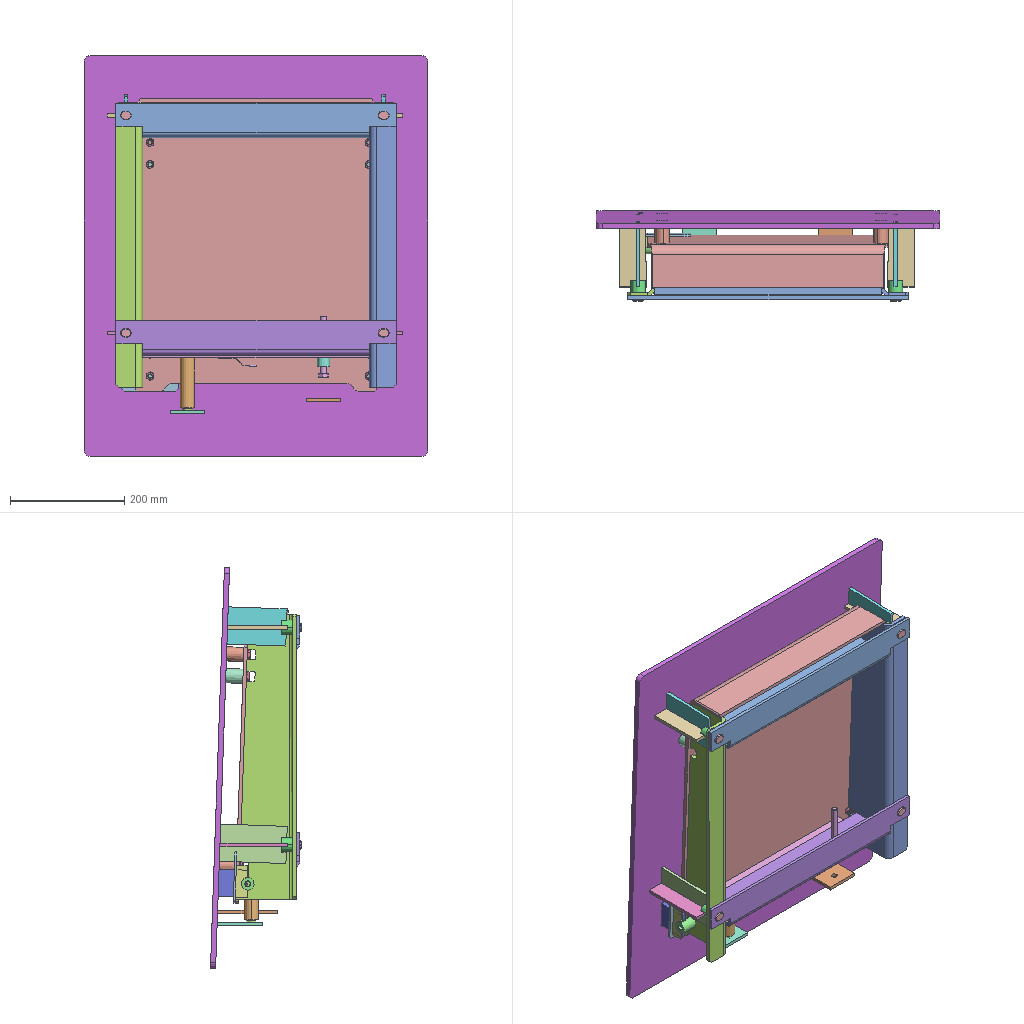Assembly | SolidWorks | 27 different items | 53 placed | box 600 x 159 x 700 mm
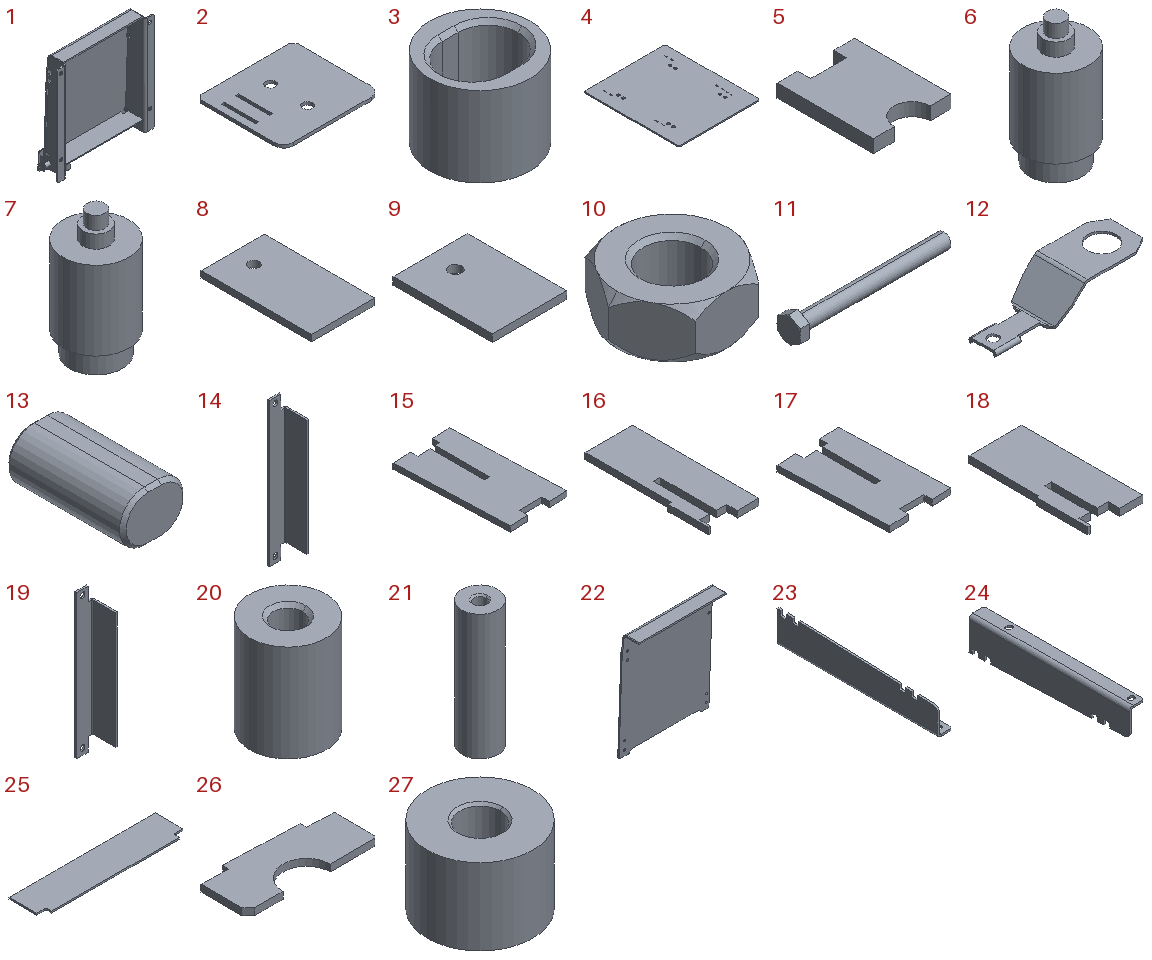Parts list (item | name | quantity | parent item | size | volume | features):
1 | (subassembly) | x1 | - | 490 x 110.428 x 539.749 mm | 2418391 mm3 | features ReferencePattern 8, LocalLPattern 4, InContextFeatHolder 2, Cut 1
2 | - | x1 | in 1 | 100 x 90 x 3.2 mm | 27363 mm3 | features FlatPattern 1, SMBaseFlange 1, SheetMetal 1
3 | - | x4 | - | 25 x 25 x 20 mm | 5055 mm3 | features Chamfer 1, Extrusion 1
4 | - | x1 | - | 600 x 700 x 9 mm | 3746150 mm3 | features Cut 3, LPattern 2, Extrusion 1, Fillet 1
5 | - | x1 | - | 47.495 x 59 x 8 mm | 19489 mm3 | features Extrusion 1
6 | - | x3 | - | 25 x 25 x 48 mm | 17814 mm3 | features ICE 3, Extrusion 1
7 | - | x5 | - | 25 x 25 x 48 mm | 17814 mm3 | features ICE 3, Extrusion 1
8 | - | x1 | - | 60 x 104.7 x 6 mm | 37221 mm3 | features FlatPattern 1, SMBaseFlange 1, SheetMetal 1
9 | - | x1 | - | 60 x 79.5 x 6 mm | 28149 mm3 | features FlatPattern 1, SMBaseFlange 1, SheetMetal 1
10 | - | x8 | in 1 | 15.011 x 13.013 x 6 mm | 641.329 mm3 | features RevCut 3, Chamfer 2, Extrusion 1, RefAxis 1
11 | - | x2 | - | 107.08 x 15.73 x 18.163 mm | 9342 mm3 | features RevCut 2, Boss 1, Chamfer 1, Extrusion 1, Fillet 1, LPattern 1, Revolution 1
12 | - | x2 | in 1 | 66.449 x 23 x 15.525 mm | 1224 mm3 | features ICE 6, EdgeFlange 2, Hem 2, FlatPattern 1, SMBaseFlange 1, SheetMetal 1
13 | - | x4 | - | 19 x 35 x 15 mm | 8232 mm3 | features Chamfer 1, Extrusion 1
14 | - | x1 | - | 60 x 80 x 490 mm | 331985 mm3 | features ICE 2, FlatPattern 1, SMBaseFlange 1, SheetMetal 1
15 | - | x2 | - | 69.342 x 126.628 x 6 mm | 43791 mm3 | features Extrusion 1, ICE 1
16 | - | x2 | - | 47.002 x 117.5 x 6 mm | 28307 mm3 | features ICE 2, Extrusion 1
17 | - | x2 | - | 68.823 x 113.082 x 6 mm | 38487 mm3 | features Extrusion 1, ICE 1
18 | - | x2 | - | 47.5 x 103.96 x 6 mm | 26008 mm3 | features ICE 2, Extrusion 1
19 | - | x1 | - | 60 x 85 x 490 mm | 343865 mm3 | features ICE 2, FlatPattern 1, SMBaseFlange 1, SheetMetal 1
20 | - | x1 | in 1 | 22 x 22 x 28 mm | 9040 mm3 | features Chamfer 1, Extrusion 1, Helix 1, ICE 1
21 | - | x1 | in 1 | 25 x 25 x 87 mm | 41273 mm3 | features Chamfer 1, Extrusion 1, Helix 1, ICE 1
22 | - | x1 | in 1 | 420 x 93.297 x 511.152 mm | 1409801 mm3 | features Cut 1, FlatPattern 1, SM3dBend 1, SMBaseFlange 1, SheetMetal 1
23 | - | x1 | in 1 | 47 x 498.4 x 101 mm | 376827 mm3 | features ICE 4, Chamfer 1, EdgeFlange 1, Fillet 1, FlatPattern 1, SMBaseFlange 1, SheetMetal 1
24 | - | x1 | in 1 | 47 x 498.4 x 101 mm | 376827 mm3 | features ICE 3, Fillet 2, Chamfer 1, EdgeFlange 1, FlatPattern 1, SMBaseFlange 1, SheetMetal 1
25 | - | x1 | in 1 | 396 x 90 x 4.5 mm | 157053 mm3 | features FlatPattern 1, SMBaseFlange 1, SheetMetal 1
26 | - | x2 | in 1 | 60 x 24.545 x 3.2 mm | 3731 mm3 | features FlatPattern 1, SMBaseFlange 1, SheetMetal 1
27 | - | x1 | in 1 | 22 x 22 x 16 mm | 5167 mm3 | features Chamfer 1, Extrusion 1, ICE 1
Mates (type | each side: item.copy, entity, surface, feature):
In the top assembly
Parallel | 22.1 face plane Base-Flange1 | 4.1 face plane Boss-Extrude1
Parallel | 22.1 face plane Sketched Bend1 | 4.1 face plane Boss-Extrude1
DistanceDim | 4.1 face plane Boss-Extrude1 | 22.1 face plane Sketched Bend1
DistanceDim | 4.1 face plane Boss-Extrude1 | 22.1 face plane Base-Flange1 | 2 times
Concentric | 4.1 face cylinder Cut-Extrude2 | 7.1 face cylinder Boss-Extrude3
Coincident | 4.1 face plane Boss-Extrude1 | 7.1 face plane Boss-Extrude3
Concentric | 4.1 face cylinder Cut-Extrude2 | 6.1 face cylinder Boss-Extrude3
Coincident | 4.1 face plane Boss-Extrude1 | 6.1 face plane Boss-Extrude3
Concentric | 4.1 face cylinder Cut-Extrude2 | 6.2 face cylinder Boss-Extrude3
Coincident | 4.1 face plane Boss-Extrude1 | 6.2 face plane Boss-Extrude3
Concentric | 4.1 face cylinder Cut-Extrude2 | 6.3 face cylinder Boss-Extrude3
Coincident | 4.1 face plane Boss-Extrude1 | 6.3 face plane Boss-Extrude3
DistanceDim | 20.1 face plane Boss-Extrude1 | 5.1 face plane Boss-Extrude1
Concentric | 20.1 face cylinder Boss-Extrude1 | 5.1 face cylinder Boss-Extrude1
Parallel | 5.1 face plane Boss-Extrude1 | 4.1 face plane Boss-Extrude1
Parallel | 23.1 face plane Base-Flange1 | 15.1 face plane Boss-Extrude1
Parallel | 23.1 face plane Edge-Flange1 | 15.1 face plane Cut-Extrude1
Coincident | 15.1 face plane Cut-Extrude1 | 16.1 face plane Boss-Extrude1
Coincident | 15.1 face plane Boss-Extrude1 | 16.1 face plane Cut-Extrude1
Coincident | 4.1 face plane LPattern4 | 17.1 face plane Boss-Extrude1 | 2 times
Coincident | 17.1 face plane Cut-Extrude1 | 18.1 face plane Boss-Extrude1
Coincident | 17.1 face plane Boss-Extrude1 | 18.1 edge
Coincident | 4.1 face plane LPattern5 | 15.2 edge
Coincident | 4.1 face plane LPattern5 | 15.2 face plane Boss-Extrude1
Coincident | 15.2 face plane Boss-Extrude1 | 16.2 edge
Coincident | 15.2 edge | 16.2 face plane Boss-Extrude1 | 2 times
Coincident | 15.2 face plane Boss-Extrude1 | 16.2 face plane Cut-Extrude1
Coincident | 4.1 face plane LPattern5 | 17.2 face plane Boss-Extrude1 | 2 times
Coincident | 17.2 face plane Boss-Extrude1 | 18.2 face plane Cut-Extrude1
Coincident | 17.2 face plane Cut-Extrude1 | 18.2 face plane Boss-Extrude1
Coincident | 24.1 face plane Base-Flange1 | 19.1 face plane Base-Flange1
Concentric | 24.1 edge | 19.1 edge
Concentric | 23.1 edge | 19.1 edge
Concentric | 24.1 face cylinder Cut-Extrude4 | 3.1 face cylinder Boss-Extrude1
Concentric | 19.1 face cylinder Cut-Extrude1 | 3.1 face cylinder Boss-Extrude1 | 2 times
Coincident | 24.1 face plane Base-Flange1 | 3.1 face plane Boss-Extrude1
Coincident | 15.2 face plane Boss-Extrude1 | 3.1 face plane Boss-Extrude1
Concentric | 3.1 face cylinder Boss-Extrude1 | 13.1 face cylinder Boss-Extrude1 | 2 times
Coincident | 23.1 face plane Base-Flange1 | 3.2 face plane Boss-Extrude1
Concentric | 19.1 face cylinder Cut-Extrude1 | 3.2 face cylinder Boss-Extrude1 | 2 times
Coincident | 23.1 face plane Base-Flange1 | 3.3 face plane Boss-Extrude1
Concentric | 23.1 face cylinder Cut-Extrude6 | 3.3 face cylinder Boss-Extrude1 | 2 times
Coincident | 24.1 face plane Base-Flange1 | 3.4 face plane Boss-Extrude1
Concentric | 24.1 face cylinder Cut-Extrude4 | 3.4 face cylinder Boss-Extrude1
Coincident | 3.2 face plane Boss-Extrude1 | 13.2 face plane Boss-Extrude1
Concentric | 23.1 face cylinder Cut-Extrude6 | 13.2 face cylinder Boss-Extrude1 | 2 times
Coincident | 3.3 face plane Boss-Extrude1 | 13.3 face plane Boss-Extrude1
Concentric | 23.1 face cylinder Cut-Extrude6 | 13.3 face cylinder Boss-Extrude1 | 2 times
Coincident | 3.4 face plane Boss-Extrude1 | 13.4 face plane Boss-Extrude1
Concentric | 24.1 face cylinder Cut-Extrude4 | 13.4 face cylinder Boss-Extrude1 | 2 times
Coincident | 24.1 face plane Base-Flange1 | 14.1 face plane Base-Flange1
Concentric | 13.4 face cylinder Boss-Extrude1 | 14.1 face cylinder Cut-Extrude1
Concentric | 13.3 face cylinder Boss-Extrude1 | 14.1 face cylinder Cut-Extrude1
Concentric | 21.1 face cylinder Boss-Extrude1 | 11.1 face cylinder BaseBody
Coincident | 21.1 face plane Cut-Extrude1 | 11.1 edge
Concentric | 27.1 face cylinder Boss-Extrude1 | 11.2 face cylinder BaseBody
Coincident | 25.1 face plane Base-Flange1 | 11.2 edge
Concentric | 21.1 face cylinder Boss-Extrude1 | 9.1 edge
DistanceDim | 21.1 face plane Boss-Extrude1 | 9.1 face plane Base-Flange1
Parallel | 24.1 face plane Edge-Flange1 | 9.1 face plane Base-Flange1
Concentric | 27.1 face cylinder Boss-Extrude1 | 8.1 face cylinder Base-Flange1
DistanceDim | 27.1 face plane Boss-Extrude1 | 8.1 face plane Base-Flange1
Parallel | 23.1 face plane Edge-Flange1 | 8.1 face plane Base-Flange1
In subassembly 1
Coincident | 22.2 face plane Sketched Bend1 | 23.2 face plane Cut-Extrude2
Parallel | 22.2 face plane Base-Flange1 | 23.2 face plane Edge-Flange1
DistanceDim | 22.2 face cylinder Base-Flange1 | 23.2 face plane Cut-Extrude4
Coincident | 22.2 face plane Sketched Bend1 | 24.2 face plane Cut-Extrude2
Parallel | 22.2 face plane Base-Flange1 | 24.2 face plane Edge-Flange1
DistanceDim | 24.2 face plane Cut-Extrude3 | 22.2 face cylinder Base-Flange1
Parallel | 23.2 face plane Edge-Flange1 | 25.2 face plane Base-Flange1
Coincident | 24.2 face plane Edge-Flange1 | 25.2 face plane Base-Flange1
DistanceDim | 25.2 edge | 22.2 face plane Sketched Bend1
DistanceDim | 24.2 face plane Edge-Flange1 | 22.2 face cylinder Base-Flange1
Coincident | 23.2 face plane Edge-Flange1 | 25.2 face plane Base-Flange1
DistanceDim | 25.2 face plane Base-Flange1 | 23.2 face plane Edge-Flange1
Coincident | 25.2 face plane Base-Flange1 | 27.2 face plane Boss-Extrude1
DistanceDim | 23.2 face plane Base-Flange1 | 27.2 face cylinder Cut-Extrude1
DistanceDim | 24.2 face plane Base-Flange1 | 27.2 face cylinder Cut-Extrude1
DistanceDim | 24.2 face plane Base-Flange1 | 21.2 face cylinder Cut-Extrude1 | 2 times
Coincident | 25.2 face plane Base-Flange1 | 21.2 face plane Boss-Extrude1
DistanceDim | 12.1 face plane Base-Flange1 | 23.2 face plane Base-Flange1
Parallel | 25.2 face plane Base-Flange1 | 12.1 face plane Base-Flange1
DistanceDim | 12.1 face plane Base-Flange1 | 24.2 face plane Base-Flange1
Coincident | 25.2 face plane Base-Flange1 | 12.2 face plane Base-Flange1
Coincident | 25.2 face plane Base-Flange1 | 12.1 face plane Base-Flange1
Coincident | 12.1 face plane Base-Flange1 | 12.2 face plane Base-Flange1
DistanceDim | 12.2 face plane Base-Flange1 | 24.2 face plane Base-Flange1
Coincident | 24.2 face plane Edge-Flange1 | 20.2 face plane Boss-Extrude1
DistanceDim | 24.2 face plane Base-Flange1 | 20.2 face cylinder Cut-Extrude1
DistanceDim | 20.2 face cylinder Cut-Extrude1 | 24.2 face cylinder Cut-Extrude4
Coincident | 22.2 face plane Sketched Bend1 | 10.1 face plane Boss-Extrude1
Concentric | 22.2 face cylinder Base-Flange1 | 10.1 face cylinder Boss-Extrude1
Parallel | 22.2 face plane Base-Flange1 | 10.1 face plane Boss-Extrude1
InPlace | 22.2 face plane Sketched Bend1 | 2.1 plane
InPlace | 22.2 face plane Base-Flange1 | 26.1 plane